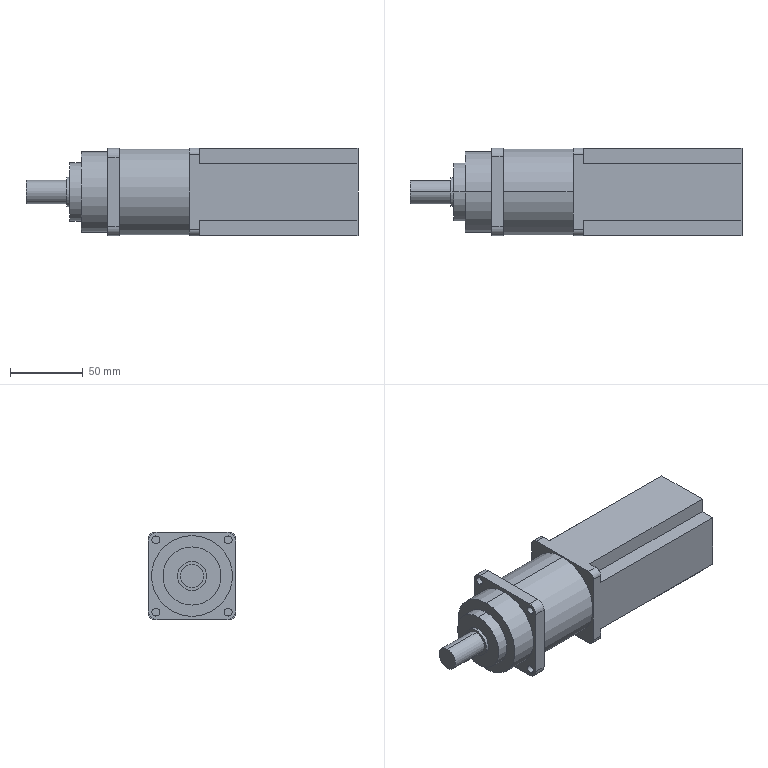Part | STEP file | 0244_101_HF-KP73BG7(1-5) | 1 solid | 54 faces | box 228 x 60 x 60 mm | volume 588290 mm3 | plane 28 | cylinder 26 | commonest cylinder face diameters 5.5 x8 9 x4 12 x4 16 x2 20 x2 40 x2